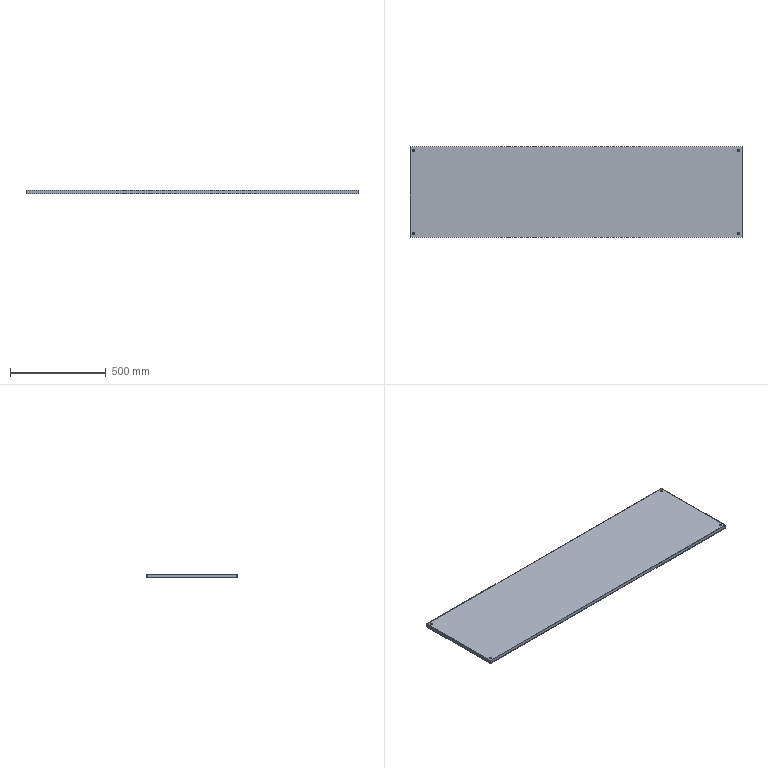Part | SolidWorks | features Extrusion 1, HoleWzd 1, ICE 1, Shell 1 | 1 solid | 32 faces | box 1736 x 471 x 20 mm | volume 1948630 mm3 | cylinder 16 | plane 16 | commonest cylinder face diameters 6.6 x8 11 x8
STEP:
#1=CARTESIAN_POINT('',(-844.5,218.5,18.));
#2=VERTEX_POINT('',#1);
#3=CARTESIAN_POINT('',(-855.5,218.5,18.));
#4=VERTEX_POINT('',#3);
#5=CARTESIAN_POINT('',(-850.,218.5,18.));
#6=DIRECTION('',(0.,0.,-1.));
#7=DIRECTION('',(-1.,0.,0.));
#8=AXIS2_PLACEMENT_3D('',#5,#6,#7);
#9=CIRCLE('',#8,5.5);
#10=EDGE_CURVE('',#2,#4,#9,.T.);
#11=ORIENTED_EDGE('',*,*,#10,.T.);
#12=CARTESIAN_POINT('',(-855.5,218.5,20.));
#13=VERTEX_POINT('',#12);
#14=CARTESIAN_POINT('',(-855.5,218.5,20.));
#15=DIRECTION('',(0.,0.,1.));
#16=VECTOR('',#15,1000.);
#17=LINE('',#14,#16);
#18=EDGE_CURVE('',#4,#13,#17,.T.);
#19=ORIENTED_EDGE('',*,*,#18,.T.);
#20=CARTESIAN_POINT('',(-844.5,218.5,20.));
#21=VERTEX_POINT('',#20);
#22=CARTESIAN_POINT('',(-850.,218.5,20.));
#23=DIRECTION('',(0.,0.,1.));
#24=DIRECTION('',(1.,0.,0.));
#25=AXIS2_PLACEMENT_3D('',#22,#23,#24);
#26=CIRCLE('',#25,5.5);
#27=EDGE_CURVE('',#13,#21,#26,.T.);
#28=ORIENTED_EDGE('',*,*,#27,.T.);
#29=CARTESIAN_POINT('',(-844.5,218.5,20.));
#30=DIRECTION('',(0.,0.,1.));
#31=VECTOR('',#30,1000.);
#32=LINE('',#29,#31);
#33=EDGE_CURVE('',#2,#21,#32,.T.);
#34=ORIENTED_EDGE('',*,*,#33,.F.);
#35=EDGE_LOOP('',(#11,#19,#28,#34));
#36=FACE_OUTER_BOUND('',#35,.T.);
#37=CARTESIAN_POINT('',(-850.,218.5,20.));
#38=DIRECTION('',(0.,0.,1.));
#39=DIRECTION('',(1.,0.,0.));
#40=AXIS2_PLACEMENT_3D('',#37,#38,#39);
#41=CYLINDRICAL_SURFACE('',#40,5.5);
#42=ADVANCED_FACE('',(#36),#41,.F.);
#43=CARTESIAN_POINT('',(-853.3,218.5,0.));
#44=VERTEX_POINT('',#43);
#45=CARTESIAN_POINT('',(-846.7,218.5,0.));
#46=VERTEX_POINT('',#45);
#47=CARTESIAN_POINT('',(-850.,218.5,0.));
#48=DIRECTION('',(0.,0.,1.));
#49=DIRECTION('',(1.,0.,0.));
#50=AXIS2_PLACEMENT_3D('',#47,#48,#49);
#51=CIRCLE('',#50,3.3);
#52=EDGE_CURVE('',#44,#46,#51,.T.);
#53=ORIENTED_EDGE('',*,*,#52,.F.);
#54=CARTESIAN_POINT('',(-853.3,218.5,2.));
#55=VERTEX_POINT('',#54);
#56=CARTESIAN_POINT('',(-853.3,218.5,20.));
#57=DIRECTION('',(0.,0.,1.));
#58=VECTOR('',#57,1000.);
#59=LINE('',#56,#58);
#60=EDGE_CURVE('',#44,#55,#59,.T.);
#61=ORIENTED_EDGE('',*,*,#60,.T.);
#62=CARTESIAN_POINT('',(-846.7,218.5,2.));
#63=VERTEX_POINT('',#62);
#64=CARTESIAN_POINT('',(-850.,218.5,2.));
#65=DIRECTION('',(0.,0.,-1.));
#66=DIRECTION('',(-1.,0.,0.));
#67=AXIS2_PLACEMENT_3D('',#64,#65,#66);
#68=CIRCLE('',#67,3.3);
#69=EDGE_CURVE('',#63,#55,#68,.T.);
#70=ORIENTED_EDGE('',*,*,#69,.F.);
#71=CARTESIAN_POINT('',(-846.7,218.5,20.));
#72=DIRECTION('',(0.,0.,1.));
#73=VECTOR('',#72,1000.);
#74=LINE('',#71,#73);
#75=EDGE_CURVE('',#46,#63,#74,.T.);
#76=ORIENTED_EDGE('',*,*,#75,.F.);
#77=EDGE_LOOP('',(#53,#61,#70,#76));
#78=FACE_OUTER_BOUND('',#77,.T.);
#79=CARTESIAN_POINT('',(-850.,218.5,20.));
#80=DIRECTION('',(0.,0.,1.));
#81=DIRECTION('',(1.,0.,0.));
#82=AXIS2_PLACEMENT_3D('',#79,#80,#81);
#83=CYLINDRICAL_SURFACE('',#82,3.3);
#84=ADVANCED_FACE('',(#78),#83,.F.);
#85=CARTESIAN_POINT('',(-844.5,-218.5,18.));
#86=VERTEX_POINT('',#85);
#87=CARTESIAN_POINT('',(-855.5,-218.5,18.));
#88=VERTEX_POINT('',#87);
#89=CARTESIAN_POINT('',(-850.,-218.5,18.));
#90=DIRECTION('',(0.,0.,-1.));
#91=DIRECTION('',(-1.,0.,0.));
#92=AXIS2_PLACEMENT_3D('',#89,#90,#91);
#93=CIRCLE('',#92,5.5);
#94=EDGE_CURVE('',#86,#88,#93,.T.);
#95=ORIENTED_EDGE('',*,*,#94,.T.);
#96=CARTESIAN_POINT('',(-855.5,-218.5,20.));
#97=VERTEX_POINT('',#96);
#98=CARTESIAN_POINT('',(-855.5,-218.5,20.));
#99=DIRECTION('',(0.,0.,1.));
#100=VECTOR('',#99,1000.);
#101=LINE('',#98,#100);
#102=EDGE_CURVE('',#88,#97,#101,.T.);
#103=ORIENTED_EDGE('',*,*,#102,.T.);
#104=CARTESIAN_POINT('',(-844.5,-218.5,20.));
#105=VERTEX_POINT('',#104);
#106=CARTESIAN_POINT('',(-850.,-218.5,20.));
#107=DIRECTION('',(0.,0.,1.));
#108=DIRECTION('',(1.,0.,0.));
#109=AXIS2_PLACEMENT_3D('',#106,#107,#108);
#110=CIRCLE('',#109,5.5);
#111=EDGE_CURVE('',#97,#105,#110,.T.);
#112=ORIENTED_EDGE('',*,*,#111,.T.);
#113=CARTESIAN_POINT('',(-844.5,-218.5,20.));
#114=DIRECTION('',(0.,0.,1.));
#115=VECTOR('',#114,1000.);
#116=LINE('',#113,#115);
#117=EDGE_CURVE('',#86,#105,#116,.T.);
#118=ORIENTED_EDGE('',*,*,#117,.F.);
#119=EDGE_LOOP('',(#95,#103,#112,#118));
#120=FACE_OUTER_BOUND('',#119,.T.);
#121=CARTESIAN_POINT('',(-850.,-218.5,20.));
#122=DIRECTION('',(0.,0.,1.));
#123=DIRECTION('',(1.,0.,0.));
#124=AXIS2_PLACEMENT_3D('',#121,#122,#123);
#125=CYLINDRICAL_SURFACE('',#124,5.5);
#126=ADVANCED_FACE('',(#120),#125,.F.);
#127=CARTESIAN_POINT('',(-853.3,-218.5,0.));
#128=VERTEX_POINT('',#127);
#129=CARTESIAN_POINT('',(-846.7,-218.5,0.));
#130=VERTEX_POINT('',#129);
#131=CARTESIAN_POINT('',(-850.,-218.5,0.));
#132=DIRECTION('',(0.,0.,1.));
#133=DIRECTION('',(1.,0.,0.));
#134=AXIS2_PLACEMENT_3D('',#131,#132,#133);
#135=CIRCLE('',#134,3.3);
#136=EDGE_CURVE('',#128,#130,#135,.T.);
#137=ORIENTED_EDGE('',*,*,#136,.F.);
#138=CARTESIAN_POINT('',(-853.3,-218.5,2.));
#139=VERTEX_POINT('',#138);
#140=CARTESIAN_POINT('',(-853.3,-218.5,20.));
#141=DIRECTION('',(0.,0.,1.));
#142=VECTOR('',#141,1000.);
#143=LINE('',#140,#142);
#144=EDGE_CURVE('',#128,#139,#143,.T.);
#145=ORIENTED_EDGE('',*,*,#144,.T.);
#146=CARTESIAN_POINT('',(-846.7,-218.5,2.));
#147=VERTEX_POINT('',#146);
#148=CARTESIAN_POINT('',(-850.,-218.5,2.));
#149=DIRECTION('',(0.,0.,-1.));
#150=DIRECTION('',(-1.,0.,0.));
#151=AXIS2_PLACEMENT_3D('',#148,#149,#150);
#152=CIRCLE('',#151,3.3);
#153=EDGE_CURVE('',#147,#139,#152,.T.);
#154=ORIENTED_EDGE('',*,*,#153,.F.);
#155=CARTESIAN_POINT('',(-846.7,-218.5,20.));
#156=DIRECTION('',(0.,0.,1.));
#157=VECTOR('',#156,1000.);
#158=LINE('',#155,#157);
#159=EDGE_CURVE('',#130,#147,#158,.T.);
#160=ORIENTED_EDGE('',*,*,#159,.F.);
#161=EDGE_LOOP('',(#137,#145,#154,#160));
#162=FACE_OUTER_BOUND('',#161,.T.);
#163=CARTESIAN_POINT('',(-850.,-218.5,20.));
#164=DIRECTION('',(0.,0.,1.));
#165=DIRECTION('',(1.,0.,0.));
#166=AXIS2_PLACEMENT_3D('',#163,#164,#165);
#167=CYLINDRICAL_SURFACE('',#166,3.3);
#168=ADVANCED_FACE('',(#162),#167,.F.);
#169=CARTESIAN_POINT('',(855.5,-218.5,18.));
#170=VERTEX_POINT('',#169);
#171=CARTESIAN_POINT('',(844.5,-218.5,18.));
#172=VERTEX_POINT('',#171);
#173=CARTESIAN_POINT('',(850.,-218.5,18.));
#174=DIRECTION('',(0.,0.,-1.));
#175=DIRECTION('',(-1.,0.,0.));
#176=AXIS2_PLACEMENT_3D('',#173,#174,#175);
#177=CIRCLE('',#176,5.5);
#178=EDGE_CURVE('',#170,#172,#177,.T.);
#179=ORIENTED_EDGE('',*,*,#178,.T.);
#180=CARTESIAN_POINT('',(844.5,-218.5,20.));
#181=VERTEX_POINT('',#180);
#182=CARTESIAN_POINT('',(844.5,-218.5,20.));
#183=DIRECTION('',(0.,0.,1.));
#184=VECTOR('',#183,1000.);
#185=LINE('',#182,#184);
#186=EDGE_CURVE('',#172,#181,#185,.T.);
#187=ORIENTED_EDGE('',*,*,#186,.T.);
#188=CARTESIAN_POINT('',(855.5,-218.5,20.));
#189=VERTEX_POINT('',#188);
#190=CARTESIAN_POINT('',(850.,-218.5,20.));
#191=DIRECTION('',(0.,0.,1.));
#192=DIRECTION('',(1.,0.,0.));
#193=AXIS2_PLACEMENT_3D('',#190,#191,#192);
#194=CIRCLE('',#193,5.5);
#195=EDGE_CURVE('',#181,#189,#194,.T.);
#196=ORIENTED_EDGE('',*,*,#195,.T.);
#197=CARTESIAN_POINT('',(855.5,-218.5,20.));
#198=DIRECTION('',(0.,0.,1.));
#199=VECTOR('',#198,1000.);
#200=LINE('',#197,#199);
#201=EDGE_CURVE('',#170,#189,#200,.T.);
#202=ORIENTED_EDGE('',*,*,#201,.F.);
#203=EDGE_LOOP('',(#179,#187,#196,#202));
#204=FACE_OUTER_BOUND('',#203,.T.);
#205=CARTESIAN_POINT('',(850.,-218.5,20.));
#206=DIRECTION('',(0.,0.,1.));
#207=DIRECTION('',(1.,0.,0.));
#208=AXIS2_PLACEMENT_3D('',#205,#206,#207);
#209=CYLINDRICAL_SURFACE('',#208,5.5);
#210=ADVANCED_FACE('',(#204),#209,.F.);
#211=CARTESIAN_POINT('',(846.7,-218.5,0.));
#212=VERTEX_POINT('',#211);
#213=CARTESIAN_POINT('',(853.3,-218.5,0.));
#214=VERTEX_POINT('',#213);
#215=CARTESIAN_POINT('',(850.,-218.5,0.));
#216=DIRECTION('',(0.,0.,1.));
#217=DIRECTION('',(1.,0.,0.));
#218=AXIS2_PLACEMENT_3D('',#215,#216,#217);
#219=CIRCLE('',#218,3.3);
#220=EDGE_CURVE('',#212,#214,#219,.T.);
#221=ORIENTED_EDGE('',*,*,#220,.F.);
#222=CARTESIAN_POINT('',(846.7,-218.5,2.));
#223=VERTEX_POINT('',#222);
#224=CARTESIAN_POINT('',(846.7,-218.5,20.));
#225=DIRECTION('',(0.,0.,1.));
#226=VECTOR('',#225,1000.);
#227=LINE('',#224,#226);
#228=EDGE_CURVE('',#212,#223,#227,.T.);
#229=ORIENTED_EDGE('',*,*,#228,.T.);
#230=CARTESIAN_POINT('',(853.3,-218.5,2.));
#231=VERTEX_POINT('',#230);
#232=CARTESIAN_POINT('',(850.,-218.5,2.));
#233=DIRECTION('',(0.,0.,-1.));
#234=DIRECTION('',(-1.,0.,0.));
#235=AXIS2_PLACEMENT_3D('',#232,#233,#234);
#236=CIRCLE('',#235,3.3);
#237=EDGE_CURVE('',#231,#223,#236,.T.);
#238=ORIENTED_EDGE('',*,*,#237,.F.);
#239=CARTESIAN_POINT('',(853.3,-218.5,20.));
#240=DIRECTION('',(0.,0.,1.));
#241=VECTOR('',#240,1000.);
#242=LINE('',#239,#241);
#243=EDGE_CURVE('',#214,#231,#242,.T.);
#244=ORIENTED_EDGE('',*,*,#243,.F.);
#245=EDGE_LOOP('',(#221,#229,#238,#244));
#246=FACE_OUTER_BOUND('',#245,.T.);
#247=CARTESIAN_POINT('',(850.,-218.5,20.));
#248=DIRECTION('',(0.,0.,1.));
#249=DIRECTION('',(1.,0.,0.));
#250=AXIS2_PLACEMENT_3D('',#247,#248,#249);
#251=CYLINDRICAL_SURFACE('',#250,3.3);
#252=ADVANCED_FACE('',(#246),#251,.F.);
#253=CARTESIAN_POINT('',(855.5,218.5,18.));
#254=VERTEX_POINT('',#253);
#255=CARTESIAN_POINT('',(844.5,218.5,18.));
#256=VERTEX_POINT('',#255);
#257=CARTESIAN_POINT('',(850.,218.5,18.));
#258=DIRECTION('',(0.,0.,-1.));
#259=DIRECTION('',(-1.,0.,0.));
#260=AXIS2_PLACEMENT_3D('',#257,#258,#259);
#261=CIRCLE('',#260,5.5);
#262=EDGE_CURVE('',#254,#256,#261,.T.);
#263=ORIENTED_EDGE('',*,*,#262,.T.);
#264=CARTESIAN_POINT('',(844.5,218.5,20.));
#265=VERTEX_POINT('',#264);
#266=CARTESIAN_POINT('',(844.5,218.5,20.));
#267=DIRECTION('',(0.,0.,1.));
#268=VECTOR('',#267,1000.);
#269=LINE('',#266,#268);
#270=EDGE_CURVE('',#256,#265,#269,.T.);
#271=ORIENTED_EDGE('',*,*,#270,.T.);
#272=CARTESIAN_POINT('',(855.5,218.5,20.));
#273=VERTEX_POINT('',#272);
#274=CARTESIAN_POINT('',(850.,218.5,20.));
#275=DIRECTION('',(0.,0.,1.));
#276=DIRECTION('',(1.,0.,0.));
#277=AXIS2_PLACEMENT_3D('',#274,#275,#276);
#278=CIRCLE('',#277,5.5);
#279=EDGE_CURVE('',#265,#273,#278,.T.);
#280=ORIENTED_EDGE('',*,*,#279,.T.);
#281=CARTESIAN_POINT('',(855.5,218.5,20.));
#282=DIRECTION('',(0.,0.,1.));
#283=VECTOR('',#282,1000.);
#284=LINE('',#281,#283);
#285=EDGE_CURVE('',#254,#273,#284,.T.);
#286=ORIENTED_EDGE('',*,*,#285,.F.);
#287=EDGE_LOOP('',(#263,#271,#280,#286));
#288=FACE_OUTER_BOUND('',#287,.T.);
#289=CARTESIAN_POINT('',(850.,218.5,20.));
#290=DIRECTION('',(0.,0.,1.));
#291=DIRECTION('',(1.,0.,0.));
#292=AXIS2_PLACEMENT_3D('',#289,#290,#291);
#293=CYLINDRICAL_SURFACE('',#292,5.5);
#294=ADVANCED_FACE('',(#288),#293,.F.);
#295=CARTESIAN_POINT('',(846.7,218.5,0.));
#296=VERTEX_POINT('',#295);
#297=CARTESIAN_POINT('',(853.3,218.5,0.));
#298=VERTEX_POINT('',#297);
#299=CARTESIAN_POINT('',(850.,218.5,0.));
#300=DIRECTION('',(0.,0.,1.));
#301=DIRECTION('',(1.,0.,0.));
#302=AXIS2_PLACEMENT_3D('',#299,#300,#301);
#303=CIRCLE('',#302,3.3);
#304=EDGE_CURVE('',#296,#298,#303,.T.);
#305=ORIENTED_EDGE('',*,*,#304,.F.);
#306=CARTESIAN_POINT('',(846.7,218.5,2.));
#307=VERTEX_POINT('',#306);
#308=CARTESIAN_POINT('',(846.7,218.5,20.));
#309=DIRECTION('',(0.,0.,1.));
#310=VECTOR('',#309,1000.);
#311=LINE('',#308,#310);
#312=EDGE_CURVE('',#296,#307,#311,.T.);
#313=ORIENTED_EDGE('',*,*,#312,.T.);
#314=CARTESIAN_POINT('',(853.3,218.5,2.));
#315=VERTEX_POINT('',#314);
#316=CARTESIAN_POINT('',(850.,218.5,2.));
#317=DIRECTION('',(0.,0.,-1.));
#318=DIRECTION('',(-1.,0.,0.));
#319=AXIS2_PLACEMENT_3D('',#316,#317,#318);
#320=CIRCLE('',#319,3.3);
#321=EDGE_CURVE('',#315,#307,#320,.T.);
#322=ORIENTED_EDGE('',*,*,#321,.F.);
#323=CARTESIAN_POINT('',(853.3,218.5,20.));
#324=DIRECTION('',(0.,0.,1.));
#325=VECTOR('',#324,1000.);
#326=LINE('',#323,#325);
#327=EDGE_CURVE('',#298,#315,#326,.T.);
#328=ORIENTED_EDGE('',*,*,#327,.F.);
#329=EDGE_LOOP('',(#305,#313,#322,#328));
#330=FACE_OUTER_BOUND('',#329,.T.);
#331=CARTESIAN_POINT('',(850.,218.5,20.));
#332=DIRECTION('',(0.,0.,1.));
#333=DIRECTION('',(1.,0.,0.));
#334=AXIS2_PLACEMENT_3D('',#331,#332,#333);
#335=CYLINDRICAL_SURFACE('',#334,3.3);
#336=ADVANCED_FACE('',(#330),#335,.F.);
#337=CARTESIAN_POINT('',(-850.,218.5,0.));
#338=DIRECTION('',(0.,0.,1.));
#339=DIRECTION('',(1.,0.,0.));
#340=AXIS2_PLACEMENT_3D('',#337,#338,#339);
#341=CIRCLE('',#340,3.3);
#342=EDGE_CURVE('',#46,#44,#341,.T.);
#343=ORIENTED_EDGE('',*,*,#342,.T.);
#344=ORIENTED_EDGE('',*,*,#52,.T.);
#345=EDGE_LOOP('',(#343,#344));
#346=FACE_BOUND('',#345,.T.);
#347=CARTESIAN_POINT('',(-850.,-218.5,0.));
#348=DIRECTION('',(0.,0.,1.));
#349=DIRECTION('',(1.,0.,0.));
#350=AXIS2_PLACEMENT_3D('',#347,#348,#349);
#351=CIRCLE('',#350,3.3);
#352=EDGE_CURVE('',#130,#128,#351,.T.);
#353=ORIENTED_EDGE('',*,*,#352,.T.);
#354=ORIENTED_EDGE('',*,*,#136,.T.);
#355=EDGE_LOOP('',(#353,#354));
#356=FACE_BOUND('',#355,.T.);
#357=CARTESIAN_POINT('',(850.,-218.5,0.));
#358=DIRECTION('',(0.,0.,1.));
#359=DIRECTION('',(1.,0.,0.));
#360=AXIS2_PLACEMENT_3D('',#357,#358,#359);
#361=CIRCLE('',#360,3.3);
#362=EDGE_CURVE('',#214,#212,#361,.T.);
#363=ORIENTED_EDGE('',*,*,#362,.T.);
#364=ORIENTED_EDGE('',*,*,#220,.T.);
#365=EDGE_LOOP('',(#363,#364));
#366=FACE_BOUND('',#365,.T.);
#367=CARTESIAN_POINT('',(850.,218.5,0.));
#368=DIRECTION('',(0.,0.,1.));
#369=DIRECTION('',(1.,0.,0.));
#370=AXIS2_PLACEMENT_3D('',#367,#368,#369);
#371=CIRCLE('',#370,3.3);
#372=EDGE_CURVE('',#298,#296,#371,.T.);
#373=ORIENTED_EDGE('',*,*,#372,.T.);
#374=ORIENTED_EDGE('',*,*,#304,.T.);
#375=EDGE_LOOP('',(#373,#374));
#376=FACE_BOUND('',#375,.T.);
#377=CARTESIAN_POINT('',(868.,-235.5,0.));
#378=VERTEX_POINT('',#377);
#379=CARTESIAN_POINT('',(868.,235.5,0.));
#380=VERTEX_POINT('',#379);
#381=CARTESIAN_POINT('',(868.,-235.5,0.));
#382=DIRECTION('',(0.,1.,0.));
#383=VECTOR('',#382,1000.);
#384=LINE('',#381,#383);
#385=EDGE_CURVE('',#378,#380,#384,.T.);
#386=ORIENTED_EDGE('',*,*,#385,.F.);
#387=CARTESIAN_POINT('',(-868.,-235.5,0.));
#388=VERTEX_POINT('',#387);
#389=CARTESIAN_POINT('',(-868.,-235.5,0.));
#390=DIRECTION('',(1.,0.,0.));
#391=VECTOR('',#390,1000.);
#392=LINE('',#389,#391);
#393=EDGE_CURVE('',#388,#378,#392,.T.);
#394=ORIENTED_EDGE('',*,*,#393,.F.);
#395=CARTESIAN_POINT('',(-868.,235.5,0.));
#396=VERTEX_POINT('',#395);
#397=CARTESIAN_POINT('',(-868.,-235.5,0.));
#398=DIRECTION('',(0.,-1.,0.));
#399=VECTOR('',#398,1000.);
#400=LINE('',#397,#399);
#401=EDGE_CURVE('',#396,#388,#400,.T.);
#402=ORIENTED_EDGE('',*,*,#401,.F.);
#403=CARTESIAN_POINT('',(-868.,235.5,0.));
#404=DIRECTION('',(-1.,0.,0.));
#405=VECTOR('',#404,1000.);
#406=LINE('',#403,#405);
#407=EDGE_CURVE('',#380,#396,#406,.T.);
#408=ORIENTED_EDGE('',*,*,#407,.F.);
#409=EDGE_LOOP('',(#386,#394,#402,#408));
#410=FACE_OUTER_BOUND('',#409,.T.);
#411=CARTESIAN_POINT('',(848.,-215.5,0.));
#412=VERTEX_POINT('',#411);
#413=CARTESIAN_POINT('',(-848.,-215.5,0.));
#414=VERTEX_POINT('',#413);
#415=CARTESIAN_POINT('',(848.,-215.5,0.));
#416=DIRECTION('',(-1.,0.,0.));
#417=VECTOR('',#416,1000.);
#418=LINE('',#415,#417);
#419=EDGE_CURVE('',#412,#414,#418,.T.);
#420=ORIENTED_EDGE('',*,*,#419,.F.);
#421=CARTESIAN_POINT('',(848.,215.5,0.));
#422=VERTEX_POINT('',#421);
#423=CARTESIAN_POINT('',(848.,-215.5,0.));
#424=DIRECTION('',(0.,1.,0.));
#425=VECTOR('',#424,1000.);
#426=LINE('',#423,#425);
#427=EDGE_CURVE('',#412,#422,#426,.T.);
#428=ORIENTED_EDGE('',*,*,#427,.T.);
#429=CARTESIAN_POINT('',(-848.,215.5,0.));
#430=VERTEX_POINT('',#429);
#431=CARTESIAN_POINT('',(848.,215.5,0.));
#432=DIRECTION('',(-1.,0.,0.));
#433=VECTOR('',#432,1000.);
#434=LINE('',#431,#433);
#435=EDGE_CURVE('',#422,#430,#434,.T.);
#436=ORIENTED_EDGE('',*,*,#435,.T.);
#437=CARTESIAN_POINT('',(-848.,-215.5,0.));
#438=DIRECTION('',(0.,1.,0.));
#439=VECTOR('',#438,1000.);
#440=LINE('',#437,#439);
#441=EDGE_CURVE('',#414,#430,#440,.T.);
#442=ORIENTED_EDGE('',*,*,#441,.F.);
#443=EDGE_LOOP('',(#420,#428,#436,#442));
#444=FACE_BOUND('',#443,.T.);
#445=CARTESIAN_POINT('',(0.,0.,0.));
#446=DIRECTION('',(0.,0.,-1.));
#447=DIRECTION('',(-1.,0.,0.));
#448=AXIS2_PLACEMENT_3D('',#445,#446,#447);
#449=PLANE('',#448);
#450=ADVANCED_FACE('',(#346,#356,#366,#376,#410,#444),#449,.T.);
#451=ORIENTED_EDGE('',*,*,#385,.T.);
#452=CARTESIAN_POINT('',(868.,235.5,20.));
#453=VERTEX_POINT('',#452);
#454=CARTESIAN_POINT('',(868.,235.5,20.));
#455=DIRECTION('',(0.,0.,-1.));
#456=VECTOR('',#455,1000.);
#457=LINE('',#454,#456);
#458=EDGE_CURVE('',#453,#380,#457,.T.);
#459=ORIENTED_EDGE('',*,*,#458,.F.);
#460=CARTESIAN_POINT('',(868.,-235.5,20.));
#461=VERTEX_POINT('',#460);
#462=CARTESIAN_POINT('',(868.,-235.5,20.));
#463=DIRECTION('',(0.,1.,0.));
#464=VECTOR('',#463,1000.);
#465=LINE('',#462,#464);
#466=EDGE_CURVE('',#461,#453,#465,.T.);
#467=ORIENTED_EDGE('',*,*,#466,.F.);
#468=CARTESIAN_POINT('',(868.,-235.5,20.));
#469=DIRECTION('',(0.,0.,-1.));
#470=VECTOR('',#469,1000.);
#471=LINE('',#468,#470);
#472=EDGE_CURVE('',#461,#378,#471,.T.);
#473=ORIENTED_EDGE('',*,*,#472,.T.);
#474=EDGE_LOOP('',(#451,#459,#467,#473));
#475=FACE_OUTER_BOUND('',#474,.T.);
#476=CARTESIAN_POINT('',(868.,-235.5,20.));
#477=DIRECTION('',(-1.,0.,0.));
#478=DIRECTION('',(0.,0.,1.));
#479=AXIS2_PLACEMENT_3D('',#476,#477,#478);
#480=PLANE('',#479);
#481=ADVANCED_FACE('',(#475),#480,.F.);
#482=ORIENTED_EDGE('',*,*,#407,.T.);
#483=CARTESIAN_POINT('',(-868.,235.5,20.));
#484=VERTEX_POINT('',#483);
#485=CARTESIAN_POINT('',(-868.,235.5,20.));
#486=DIRECTION('',(0.,0.,-1.));
#487=VECTOR('',#486,1000.);
#488=LINE('',#485,#487);
#489=EDGE_CURVE('',#484,#396,#488,.T.);
#490=ORIENTED_EDGE('',*,*,#489,.F.);
#491=CARTESIAN_POINT('',(-868.,235.5,20.));
#492=DIRECTION('',(-1.,0.,0.));
#493=VECTOR('',#492,1000.);
#494=LINE('',#491,#493);
#495=EDGE_CURVE('',#453,#484,#494,.T.);
#496=ORIENTED_EDGE('',*,*,#495,.F.);
#497=ORIENTED_EDGE('',*,*,#458,.T.);
#498=EDGE_LOOP('',(#482,#490,#496,#497));
#499=FACE_OUTER_BOUND('',#498,.T.);
#500=CARTESIAN_POINT('',(-868.,235.5,20.));
#501=DIRECTION('',(0.,-1.,0.));
#502=DIRECTION('',(0.,0.,-1.));
#503=AXIS2_PLACEMENT_3D('',#500,#501,#502);
#504=PLANE('',#503);
#505=ADVANCED_FACE('',(#499),#504,.F.);
#506=ORIENTED_EDGE('',*,*,#401,.T.);
#507=CARTESIAN_POINT('',(-868.,-235.5,20.));
#508=VERTEX_POINT('',#507);
#509=CARTESIAN_POINT('',(-868.,-235.5,20.));
#510=DIRECTION('',(0.,0.,-1.));
#511=VECTOR('',#510,1000.);
#512=LINE('',#509,#511);
#513=EDGE_CURVE('',#508,#388,#512,.T.);
#514=ORIENTED_EDGE('',*,*,#513,.F.);
#515=CARTESIAN_POINT('',(-868.,-235.5,20.));
#516=DIRECTION('',(0.,-1.,0.));
#517=VECTOR('',#516,1000.);
#518=LINE('',#515,#517);
#519=EDGE_CURVE('',#484,#508,#518,.T.);
#520=ORIENTED_EDGE('',*,*,#519,.F.);
#521=ORIENTED_EDGE('',*,*,#489,.T.);
#522=EDGE_LOOP('',(#506,#514,#520,#521));
#523=FACE_OUTER_BOUND('',#522,.T.);
#524=CARTESIAN_POINT('',(-868.,-235.5,20.));
#525=DIRECTION('',(1.,0.,0.));
#526=DIRECTION('',(0.,0.,-1.));
#527=AXIS2_PLACEMENT_3D('',#524,#525,#526);
#528=PLANE('',#527);
#529=ADVANCED_FACE('',(#523),#528,.F.);
#530=ORIENTED_EDGE('',*,*,#393,.T.);
#531=ORIENTED_EDGE('',*,*,#472,.F.);
#532=CARTESIAN_POINT('',(-868.,-235.5,20.));
#533=DIRECTION('',(1.,0.,0.));
#534=VECTOR('',#533,1000.);
#535=LINE('',#532,#534);
#536=EDGE_CURVE('',#508,#461,#535,.T.);
#537=ORIENTED_EDGE('',*,*,#536,.F.);
#538=ORIENTED_EDGE('',*,*,#513,.T.);
#539=EDGE_LOOP('',(#530,#531,#537,#538));
#540=FACE_OUTER_BOUND('',#539,.T.);
#541=CARTESIAN_POINT('',(-868.,-235.5,20.));
#542=DIRECTION('',(0.,1.,0.));
#543=DIRECTION('',(0.,0.,1.));
#544=AXIS2_PLACEMENT_3D('',#541,#542,#543);
#545=PLANE('',#544);
#546=ADVANCED_FACE('',(#540),#545,.F.);
#547=CARTESIAN_POINT('',(-850.,218.5,20.));
#548=DIRECTION('',(0.,0.,1.));
#549=DIRECTION('',(1.,0.,0.));
#550=AXIS2_PLACEMENT_3D('',#547,#548,#549);
#551=CIRCLE('',#550,5.5);
#552=EDGE_CURVE('',#21,#13,#551,.T.);
#553=ORIENTED_EDGE('',*,*,#552,.F.);
#554=ORIENTED_EDGE('',*,*,#27,.F.);
#555=EDGE_LOOP('',(#553,#554));
#556=FACE_BOUND('',#555,.T.);
#557=CARTESIAN_POINT('',(-850.,-218.5,20.));
#558=DIRECTION('',(0.,0.,1.));
#559=DIRECTION('',(1.,0.,0.));
#560=AXIS2_PLACEMENT_3D('',#557,#558,#559);
#561=CIRCLE('',#560,5.5);
#562=EDGE_CURVE('',#105,#97,#561,.T.);
#563=ORIENTED_EDGE('',*,*,#562,.F.);
#564=ORIENTED_EDGE('',*,*,#111,.F.);
#565=EDGE_LOOP('',(#563,#564));
#566=FACE_BOUND('',#565,.T.);
#567=CARTESIAN_POINT('',(850.,-218.5,20.));
#568=DIRECTION('',(0.,0.,1.));
#569=DIRECTION('',(1.,0.,0.));
#570=AXIS2_PLACEMENT_3D('',#567,#568,#569);
#571=CIRCLE('',#570,5.5);
#572=EDGE_CURVE('',#189,#181,#571,.T.);
#573=ORIENTED_EDGE('',*,*,#572,.F.);
#574=ORIENTED_EDGE('',*,*,#195,.F.);
#575=EDGE_LOOP('',(#573,#574));
#576=FACE_BOUND('',#575,.T.);
#577=CARTESIAN_POINT('',(850.,218.5,20.));
#578=DIRECTION('',(0.,0.,1.));
#579=DIRECTION('',(1.,0.,0.));
#580=AXIS2_PLACEMENT_3D('',#577,#578,#579);
#581=CIRCLE('',#580,5.5);
#582=EDGE_CURVE('',#273,#265,#581,.T.);
#583=ORIENTED_EDGE('',*,*,#582,.F.);
#584=ORIENTED_EDGE('',*,*,#279,.F.);
#585=EDGE_LOOP('',(#583,#584));
#586=FACE_BOUND('',#585,.T.);
#587=ORIENTED_EDGE('',*,*,#466,.T.);
#588=ORIENTED_EDGE('',*,*,#495,.T.);
#589=ORIENTED_EDGE('',*,*,#519,.T.);
#590=ORIENTED_EDGE('',*,*,#536,.T.);
#591=EDGE_LOOP('',(#587,#588,#589,#590));
#592=FACE_OUTER_BOUND('',#591,.T.);
#593=CARTESIAN_POINT('',(0.,0.,20.));
#594=DIRECTION('',(0.,0.,-1.));
#595=DIRECTION('',(-1.,0.,0.));
#596=AXIS2_PLACEMENT_3D('',#593,#594,#595);
#597=PLANE('',#596);
#598=ADVANCED_FACE('',(#556,#566,#576,#586,#592),#597,.F.);
#599=ORIENTED_EDGE('',*,*,#427,.F.);
#600=CARTESIAN_POINT('',(848.,-215.5,2.));
#601=VERTEX_POINT('',#600);
#602=CARTESIAN_POINT('',(848.,-215.5,2.));
#603=DIRECTION('',(0.,0.,-1.));
#604=VECTOR('',#603,1000.);
#605=LINE('',#602,#604);
#606=EDGE_CURVE('',#601,#412,#605,.T.);
#607=ORIENTED_EDGE('',*,*,#606,.F.);
#608=CARTESIAN_POINT('',(848.,215.5,2.));
#609=VERTEX_POINT('',#608);
#610=CARTESIAN_POINT('',(848.,-215.5,2.));
#611=DIRECTION('',(0.,1.,0.));
#612=VECTOR('',#611,1000.);
#613=LINE('',#610,#612);
#614=EDGE_CURVE('',#601,#609,#613,.T.);
#615=ORIENTED_EDGE('',*,*,#614,.T.);
#616=CARTESIAN_POINT('',(848.,215.5,2.));
#617=DIRECTION('',(0.,0.,-1.));
#618=VECTOR('',#617,1000.);
#619=LINE('',#616,#618);
#620=EDGE_CURVE('',#609,#422,#619,.T.);
#621=ORIENTED_EDGE('',*,*,#620,.T.);
#622=EDGE_LOOP('',(#599,#607,#615,#621));
#623=FACE_OUTER_BOUND('',#622,.T.);
#624=CARTESIAN_POINT('',(848.,-215.5,2.));
#625=DIRECTION('',(-1.,0.,0.));
#626=DIRECTION('',(0.,0.,1.));
#627=AXIS2_PLACEMENT_3D('',#624,#625,#626);
#628=PLANE('',#627);
#629=ADVANCED_FACE('',(#623),#628,.T.);
#630=ORIENTED_EDGE('',*,*,#435,.F.);
#631=ORIENTED_EDGE('',*,*,#620,.F.);
#632=CARTESIAN_POINT('',(-848.,215.5,2.));
#633=VERTEX_POINT('',#632);
#634=CARTESIAN_POINT('',(848.,215.5,2.));
#635=DIRECTION('',(-1.,0.,0.));
#636=VECTOR('',#635,1000.);
#637=LINE('',#634,#636);
#638=EDGE_CURVE('',#609,#633,#637,.T.);
#639=ORIENTED_EDGE('',*,*,#638,.T.);
#640=CARTESIAN_POINT('',(-848.,215.5,2.));
#641=DIRECTION('',(0.,0.,-1.));
#642=VECTOR('',#641,1000.);
#643=LINE('',#640,#642);
#644=EDGE_CURVE('',#633,#430,#643,.T.);
#645=ORIENTED_EDGE('',*,*,#644,.T.);
#646=EDGE_LOOP('',(#630,#631,#639,#645));
#647=FACE_OUTER_BOUND('',#646,.T.);
#648=CARTESIAN_POINT('',(848.,215.5,2.));
#649=DIRECTION('',(0.,-1.,0.));
#650=DIRECTION('',(0.,0.,-1.));
#651=AXIS2_PLACEMENT_3D('',#648,#649,#650);
#652=PLANE('',#651);
#653=ADVANCED_FACE('',(#647),#652,.T.);
#654=ORIENTED_EDGE('',*,*,#441,.T.);
#655=ORIENTED_EDGE('',*,*,#644,.F.);
#656=CARTESIAN_POINT('',(-848.,-215.5,2.));
#657=VERTEX_POINT('',#656);
#658=CARTESIAN_POINT('',(-848.,-215.5,2.));
#659=DIRECTION('',(0.,1.,0.));
#660=VECTOR('',#659,1000.);
#661=LINE('',#658,#660);
#662=EDGE_CURVE('',#657,#633,#661,.T.);
#663=ORIENTED_EDGE('',*,*,#662,.F.);
#664=CARTESIAN_POINT('',(-848.,-215.5,2.));
#665=DIRECTION('',(0.,0.,-1.));
#666=VECTOR('',#665,1000.);
#667=LINE('',#664,#666);
#668=EDGE_CURVE('',#657,#414,#667,.T.);
#669=ORIENTED_EDGE('',*,*,#668,.T.);
#670=EDGE_LOOP('',(#654,#655,#663,#669));
#671=FACE_OUTER_BOUND('',#670,.T.);
#672=CARTESIAN_POINT('',(-848.,-215.5,2.));
#673=DIRECTION('',(-1.,0.,0.));
#674=DIRECTION('',(0.,0.,1.));
#675=AXIS2_PLACEMENT_3D('',#672,#673,#674);
#676=PLANE('',#675);
#677=ADVANCED_FACE('',(#671),#676,.F.);
#678=ORIENTED_EDGE('',*,*,#419,.T.);
#679=ORIENTED_EDGE('',*,*,#668,.F.);
#680=CARTESIAN_POINT('',(848.,-215.5,2.));
#681=DIRECTION('',(-1.,0.,0.));
#682=VECTOR('',#681,1000.);
#683=LINE('',#680,#682);
#684=EDGE_CURVE('',#601,#657,#683,.T.);
#685=ORIENTED_EDGE('',*,*,#684,.F.);
#686=ORIENTED_EDGE('',*,*,#606,.T.);
#687=EDGE_LOOP('',(#678,#679,#685,#686));
#688=FACE_OUTER_BOUND('',#687,.T.);
#689=CARTESIAN_POINT('',(848.,-215.5,2.));
#690=DIRECTION('',(0.,-1.,0.));
#691=DIRECTION('',(0.,0.,-1.));
#692=AXIS2_PLACEMENT_3D('',#689,#690,#691);
#693=PLANE('',#692);
#694=ADVANCED_FACE('',(#688),#693,.F.);
#695=ORIENTED_EDGE('',*,*,#69,.T.);
#696=CARTESIAN_POINT('',(-850.,218.5,2.));
#697=DIRECTION('',(0.,0.,-1.));
#698=DIRECTION('',(-1.,0.,0.));
#699=AXIS2_PLACEMENT_3D('',#696,#697,#698);
#700=CIRCLE('',#699,3.3);
#701=EDGE_CURVE('',#55,#63,#700,.T.);
#702=ORIENTED_EDGE('',*,*,#701,.T.);
#703=EDGE_LOOP('',(#695,#702));
#704=FACE_BOUND('',#703,.T.);
#705=ORIENTED_EDGE('',*,*,#153,.T.);
#706=CARTESIAN_POINT('',(-850.,-218.5,2.));
#707=DIRECTION('',(0.,0.,-1.));
#708=DIRECTION('',(-1.,0.,0.));
#709=AXIS2_PLACEMENT_3D('',#706,#707,#708);
#710=CIRCLE('',#709,3.3);
#711=EDGE_CURVE('',#139,#147,#710,.T.);
#712=ORIENTED_EDGE('',*,*,#711,.T.);
#713=EDGE_LOOP('',(#705,#712));
#714=FACE_BOUND('',#713,.T.);
#715=ORIENTED_EDGE('',*,*,#237,.T.);
#716=CARTESIAN_POINT('',(850.,-218.5,2.));
#717=DIRECTION('',(0.,0.,-1.));
#718=DIRECTION('',(-1.,0.,0.));
#719=AXIS2_PLACEMENT_3D('',#716,#717,#718);
#720=CIRCLE('',#719,3.3);
#721=EDGE_CURVE('',#223,#231,#720,.T.);
#722=ORIENTED_EDGE('',*,*,#721,.T.);
#723=EDGE_LOOP('',(#715,#722));
#724=FACE_BOUND('',#723,.T.);
#725=ORIENTED_EDGE('',*,*,#321,.T.);
#726=CARTESIAN_POINT('',(850.,218.5,2.));
#727=DIRECTION('',(0.,0.,-1.));
#728=DIRECTION('',(-1.,0.,0.));
#729=AXIS2_PLACEMENT_3D('',#726,#727,#728);
#730=CIRCLE('',#729,3.3);
#731=EDGE_CURVE('',#307,#315,#730,.T.);
#732=ORIENTED_EDGE('',*,*,#731,.T.);
#733=EDGE_LOOP('',(#725,#732));
#734=FACE_BOUND('',#733,.T.);
#735=CARTESIAN_POINT('',(866.,-233.5,2.));
#736=VERTEX_POINT('',#735);
#737=CARTESIAN_POINT('',(866.,233.5,2.));
#738=VERTEX_POINT('',#737);
#739=CARTESIAN_POINT('',(866.,0.,2.));
#740=DIRECTION('',(0.,1.,0.));
#741=VECTOR('',#740,1000.);
#742=LINE('',#739,#741);
#743=EDGE_CURVE('',#736,#738,#742,.T.);
#744=ORIENTED_EDGE('',*,*,#743,.T.);
#745=CARTESIAN_POINT('',(-866.,233.5,2.));
#746=VERTEX_POINT('',#745);
#747=CARTESIAN_POINT('',(0.,233.5,2.));
#748=DIRECTION('',(-1.,0.,0.));
#749=VECTOR('',#748,1000.);
#750=LINE('',#747,#749);
#751=EDGE_CURVE('',#738,#746,#750,.T.);
#752=ORIENTED_EDGE('',*,*,#751,.T.);
#753=CARTESIAN_POINT('',(-866.,-233.5,2.));
#754=VERTEX_POINT('',#753);
#755=CARTESIAN_POINT('',(-866.,0.,2.));
#756=DIRECTION('',(0.,-1.,0.));
#757=VECTOR('',#756,1000.);
#758=LINE('',#755,#757);
#759=EDGE_CURVE('',#746,#754,#758,.T.);
#760=ORIENTED_EDGE('',*,*,#759,.T.);
#761=CARTESIAN_POINT('',(0.,-233.5,2.));
#762=DIRECTION('',(1.,0.,0.));
#763=VECTOR('',#762,1000.);
#764=LINE('',#761,#763);
#765=EDGE_CURVE('',#754,#736,#764,.T.);
#766=ORIENTED_EDGE('',*,*,#765,.T.);
#767=EDGE_LOOP('',(#744,#752,#760,#766));
#768=FACE_OUTER_BOUND('',#767,.T.);
#769=ORIENTED_EDGE('',*,*,#684,.T.);
#770=ORIENTED_EDGE('',*,*,#662,.T.);
#771=ORIENTED_EDGE('',*,*,#638,.F.);
#772=ORIENTED_EDGE('',*,*,#614,.F.);
#773=EDGE_LOOP('',(#769,#770,#771,#772));
#774=FACE_BOUND('',#773,.T.);
#775=CARTESIAN_POINT('',(0.,0.,2.));
#776=DIRECTION('',(0.,0.,-1.));
#777=DIRECTION('',(-1.,0.,0.));
#778=AXIS2_PLACEMENT_3D('',#775,#776,#777);
#779=PLANE('',#778);
#780=ADVANCED_FACE('',(#704,#714,#724,#734,#768,#774),#779,.F.);
#781=ORIENTED_EDGE('',*,*,#743,.F.);
#782=CARTESIAN_POINT('',(866.,-233.5,18.));
#783=VERTEX_POINT('',#782);
#784=CARTESIAN_POINT('',(866.,-233.5,20.));
#785=DIRECTION('',(0.,0.,-1.));
#786=VECTOR('',#785,1000.);
#787=LINE('',#784,#786);
#788=EDGE_CURVE('',#783,#736,#787,.T.);
#789=ORIENTED_EDGE('',*,*,#788,.F.);
#790=CARTESIAN_POINT('',(866.,233.5,18.));
#791=VERTEX_POINT('',#790);
#792=CARTESIAN_POINT('',(866.,0.,18.));
#793=DIRECTION('',(0.,1.,0.));
#794=VECTOR('',#793,1000.);
#795=LINE('',#792,#794);
#796=EDGE_CURVE('',#783,#791,#795,.T.);
#797=ORIENTED_EDGE('',*,*,#796,.T.);
#798=CARTESIAN_POINT('',(866.,233.5,20.));
#799=DIRECTION('',(0.,0.,-1.));
#800=VECTOR('',#799,1000.);
#801=LINE('',#798,#800);
#802=EDGE_CURVE('',#791,#738,#801,.T.);
#803=ORIENTED_EDGE('',*,*,#802,.T.);
#804=EDGE_LOOP('',(#781,#789,#797,#803));
#805=FACE_OUTER_BOUND('',#804,.T.);
#806=CARTESIAN_POINT('',(866.,-235.5,20.));
#807=DIRECTION('',(-1.,0.,0.));
#808=DIRECTION('',(0.,0.,1.));
#809=AXIS2_PLACEMENT_3D('',#806,#807,#808);
#810=PLANE('',#809);
#811=ADVANCED_FACE('',(#805),#810,.T.);
#812=ORIENTED_EDGE('',*,*,#751,.F.);
#813=ORIENTED_EDGE('',*,*,#802,.F.);
#814=CARTESIAN_POINT('',(-866.,233.5,18.));
#815=VERTEX_POINT('',#814);
#816=CARTESIAN_POINT('',(0.,233.5,18.));
#817=DIRECTION('',(-1.,0.,0.));
#818=VECTOR('',#817,1000.);
#819=LINE('',#816,#818);
#820=EDGE_CURVE('',#791,#815,#819,.T.);
#821=ORIENTED_EDGE('',*,*,#820,.T.);
#822=CARTESIAN_POINT('',(-866.,233.5,20.));
#823=DIRECTION('',(0.,0.,-1.));
#824=VECTOR('',#823,1000.);
#825=LINE('',#822,#824);
#826=EDGE_CURVE('',#815,#746,#825,.T.);
#827=ORIENTED_EDGE('',*,*,#826,.T.);
#828=EDGE_LOOP('',(#812,#813,#821,#827));
#829=FACE_OUTER_BOUND('',#828,.T.);
#830=CARTESIAN_POINT('',(-868.,233.5,20.));
#831=DIRECTION('',(0.,-1.,0.));
#832=DIRECTION('',(0.,0.,-1.));
#833=AXIS2_PLACEMENT_3D('',#830,#831,#832);
#834=PLANE('',#833);
#835=ADVANCED_FACE('',(#829),#834,.T.);
#836=ORIENTED_EDGE('',*,*,#759,.F.);
#837=ORIENTED_EDGE('',*,*,#826,.F.);
#838=CARTESIAN_POINT('',(-866.,-233.5,18.));
#839=VERTEX_POINT('',#838);
#840=CARTESIAN_POINT('',(-866.,0.,18.));
#841=DIRECTION('',(0.,-1.,0.));
#842=VECTOR('',#841,1000.);
#843=LINE('',#840,#842);
#844=EDGE_CURVE('',#815,#839,#843,.T.);
#845=ORIENTED_EDGE('',*,*,#844,.T.);
#846=CARTESIAN_POINT('',(-866.,-233.5,20.));
#847=DIRECTION('',(0.,0.,-1.));
#848=VECTOR('',#847,1000.);
#849=LINE('',#846,#848);
#850=EDGE_CURVE('',#839,#754,#849,.T.);
#851=ORIENTED_EDGE('',*,*,#850,.T.);
#852=EDGE_LOOP('',(#836,#837,#845,#851));
#853=FACE_OUTER_BOUND('',#852,.T.);
#854=CARTESIAN_POINT('',(-866.,-235.5,20.));
#855=DIRECTION('',(1.,0.,0.));
#856=DIRECTION('',(0.,0.,-1.));
#857=AXIS2_PLACEMENT_3D('',#854,#855,#856);
#858=PLANE('',#857);
#859=ADVANCED_FACE('',(#853),#858,.T.);
#860=ORIENTED_EDGE('',*,*,#765,.F.);
#861=ORIENTED_EDGE('',*,*,#850,.F.);
#862=CARTESIAN_POINT('',(0.,-233.5,18.));
#863=DIRECTION('',(1.,0.,0.));
#864=VECTOR('',#863,1000.);
#865=LINE('',#862,#864);
#866=EDGE_CURVE('',#839,#783,#865,.T.);
#867=ORIENTED_EDGE('',*,*,#866,.T.);
#868=ORIENTED_EDGE('',*,*,#788,.T.);
#869=EDGE_LOOP('',(#860,#861,#867,#868));
#870=FACE_OUTER_BOUND('',#869,.T.);
#871=CARTESIAN_POINT('',(-868.,-233.5,20.));
#872=DIRECTION('',(0.,1.,0.));
#873=DIRECTION('',(0.,0.,1.));
#874=AXIS2_PLACEMENT_3D('',#871,#872,#873);
#875=PLANE('',#874);
#876=ADVANCED_FACE('',(#870),#875,.T.);
#877=ORIENTED_EDGE('',*,*,#10,.F.);
#878=CARTESIAN_POINT('',(-850.,218.5,18.));
#879=DIRECTION('',(0.,0.,-1.));
#880=DIRECTION('',(-1.,0.,0.));
#881=AXIS2_PLACEMENT_3D('',#878,#879,#880);
#882=CIRCLE('',#881,5.5);
#883=EDGE_CURVE('',#4,#2,#882,.T.);
#884=ORIENTED_EDGE('',*,*,#883,.F.);
#885=EDGE_LOOP('',(#877,#884));
#886=FACE_BOUND('',#885,.T.);
#887=ORIENTED_EDGE('',*,*,#94,.F.);
#888=CARTESIAN_POINT('',(-850.,-218.5,18.));
#889=DIRECTION('',(0.,0.,-1.));
#890=DIRECTION('',(-1.,0.,0.));
#891=AXIS2_PLACEMENT_3D('',#888,#889,#890);
#892=CIRCLE('',#891,5.5);
#893=EDGE_CURVE('',#88,#86,#892,.T.);
#894=ORIENTED_EDGE('',*,*,#893,.F.);
#895=EDGE_LOOP('',(#887,#894));
#896=FACE_BOUND('',#895,.T.);
#897=ORIENTED_EDGE('',*,*,#178,.F.);
#898=CARTESIAN_POINT('',(850.,-218.5,18.));
#899=DIRECTION('',(0.,0.,-1.));
#900=DIRECTION('',(-1.,0.,0.));
#901=AXIS2_PLACEMENT_3D('',#898,#899,#900);
#902=CIRCLE('',#901,5.5);
#903=EDGE_CURVE('',#172,#170,#902,.T.);
#904=ORIENTED_EDGE('',*,*,#903,.F.);
#905=EDGE_LOOP('',(#897,#904));
#906=FACE_BOUND('',#905,.T.);
#907=ORIENTED_EDGE('',*,*,#262,.F.);
#908=CARTESIAN_POINT('',(850.,218.5,18.));
#909=DIRECTION('',(0.,0.,-1.));
#910=DIRECTION('',(-1.,0.,0.));
#911=AXIS2_PLACEMENT_3D('',#908,#909,#910);
#912=CIRCLE('',#911,5.5);
#913=EDGE_CURVE('',#256,#254,#912,.T.);
#914=ORIENTED_EDGE('',*,*,#913,.F.);
#915=EDGE_LOOP('',(#907,#914));
#916=FACE_BOUND('',#915,.T.);
#917=ORIENTED_EDGE('',*,*,#796,.F.);
#918=ORIENTED_EDGE('',*,*,#866,.F.);
#919=ORIENTED_EDGE('',*,*,#844,.F.);
#920=ORIENTED_EDGE('',*,*,#820,.F.);
#921=EDGE_LOOP('',(#917,#918,#919,#920));
#922=FACE_OUTER_BOUND('',#921,.T.);
#923=CARTESIAN_POINT('',(0.,0.,18.));
#924=DIRECTION('',(0.,0.,-1.));
#925=DIRECTION('',(-1.,0.,0.));
#926=AXIS2_PLACEMENT_3D('',#923,#924,#925);
#927=PLANE('',#926);
#928=ADVANCED_FACE('',(#886,#896,#906,#916,#922),#927,.T.);
#929=ORIENTED_EDGE('',*,*,#312,.F.);
#930=ORIENTED_EDGE('',*,*,#372,.F.);
#931=ORIENTED_EDGE('',*,*,#327,.T.);
#932=ORIENTED_EDGE('',*,*,#731,.F.);
#933=EDGE_LOOP('',(#929,#930,#931,#932));
#934=FACE_OUTER_BOUND('',#933,.T.);
#935=CARTESIAN_POINT('',(850.,218.5,20.));
#936=DIRECTION('',(0.,0.,1.));
#937=DIRECTION('',(1.,0.,0.));
#938=AXIS2_PLACEMENT_3D('',#935,#936,#937);
#939=CYLINDRICAL_SURFACE('',#938,3.3);
#940=ADVANCED_FACE('',(#934),#939,.F.);
#941=ORIENTED_EDGE('',*,*,#270,.F.);
#942=ORIENTED_EDGE('',*,*,#913,.T.);
#943=ORIENTED_EDGE('',*,*,#285,.T.);
#944=ORIENTED_EDGE('',*,*,#582,.T.);
#945=EDGE_LOOP('',(#941,#942,#943,#944));
#946=FACE_OUTER_BOUND('',#945,.T.);
#947=CARTESIAN_POINT('',(850.,218.5,20.));
#948=DIRECTION('',(0.,0.,1.));
#949=DIRECTION('',(1.,0.,0.));
#950=AXIS2_PLACEMENT_3D('',#947,#948,#949);
#951=CYLINDRICAL_SURFACE('',#950,5.5);
#952=ADVANCED_FACE('',(#946),#951,.F.);
#953=ORIENTED_EDGE('',*,*,#228,.F.);
#954=ORIENTED_EDGE('',*,*,#362,.F.);
#955=ORIENTED_EDGE('',*,*,#243,.T.);
#956=ORIENTED_EDGE('',*,*,#721,.F.);
#957=EDGE_LOOP('',(#953,#954,#955,#956));
#958=FACE_OUTER_BOUND('',#957,.T.);
#959=CARTESIAN_POINT('',(850.,-218.5,20.));
#960=DIRECTION('',(0.,0.,1.));
#961=DIRECTION('',(1.,0.,0.));
#962=AXIS2_PLACEMENT_3D('',#959,#960,#961);
#963=CYLINDRICAL_SURFACE('',#962,3.3);
#964=ADVANCED_FACE('',(#958),#963,.F.);
#965=ORIENTED_EDGE('',*,*,#186,.F.);
#966=ORIENTED_EDGE('',*,*,#903,.T.);
#967=ORIENTED_EDGE('',*,*,#201,.T.);
#968=ORIENTED_EDGE('',*,*,#572,.T.);
#969=EDGE_LOOP('',(#965,#966,#967,#968));
#970=FACE_OUTER_BOUND('',#969,.T.);
#971=CARTESIAN_POINT('',(850.,-218.5,20.));
#972=DIRECTION('',(0.,0.,1.));
#973=DIRECTION('',(1.,0.,0.));
#974=AXIS2_PLACEMENT_3D('',#971,#972,#973);
#975=CYLINDRICAL_SURFACE('',#974,5.5);
#976=ADVANCED_FACE('',(#970),#975,.F.);
#977=ORIENTED_EDGE('',*,*,#144,.F.);
#978=ORIENTED_EDGE('',*,*,#352,.F.);
#979=ORIENTED_EDGE('',*,*,#159,.T.);
#980=ORIENTED_EDGE('',*,*,#711,.F.);
#981=EDGE_LOOP('',(#977,#978,#979,#980));
#982=FACE_OUTER_BOUND('',#981,.T.);
#983=CARTESIAN_POINT('',(-850.,-218.5,20.));
#984=DIRECTION('',(0.,0.,1.));
#985=DIRECTION('',(1.,0.,0.));
#986=AXIS2_PLACEMENT_3D('',#983,#984,#985);
#987=CYLINDRICAL_SURFACE('',#986,3.3);
#988=ADVANCED_FACE('',(#982),#987,.F.);
#989=ORIENTED_EDGE('',*,*,#102,.F.);
#990=ORIENTED_EDGE('',*,*,#893,.T.);
#991=ORIENTED_EDGE('',*,*,#117,.T.);
#992=ORIENTED_EDGE('',*,*,#562,.T.);
#993=EDGE_LOOP('',(#989,#990,#991,#992));
#994=FACE_OUTER_BOUND('',#993,.T.);
#995=CARTESIAN_POINT('',(-850.,-218.5,20.));
#996=DIRECTION('',(0.,0.,1.));
#997=DIRECTION('',(1.,0.,0.));
#998=AXIS2_PLACEMENT_3D('',#995,#996,#997);
#999=CYLINDRICAL_SURFACE('',#998,5.5);
#1000=ADVANCED_FACE('',(#994),#999,.F.);
#1001=ORIENTED_EDGE('',*,*,#60,.F.);
#1002=ORIENTED_EDGE('',*,*,#342,.F.);
#1003=ORIENTED_EDGE('',*,*,#75,.T.);
#1004=ORIENTED_EDGE('',*,*,#701,.F.);
#1005=EDGE_LOOP('',(#1001,#1002,#1003,#1004));
#1006=FACE_OUTER_BOUND('',#1005,.T.);
#1007=CARTESIAN_POINT('',(-850.,218.5,20.));
#1008=DIRECTION('',(0.,0.,1.));
#1009=DIRECTION('',(1.,0.,0.));
#1010=AXIS2_PLACEMENT_3D('',#1007,#1008,#1009);
#1011=CYLINDRICAL_SURFACE('',#1010,3.3);
#1012=ADVANCED_FACE('',(#1006),#1011,.F.);
#1013=ORIENTED_EDGE('',*,*,#18,.F.);
#1014=ORIENTED_EDGE('',*,*,#883,.T.);
#1015=ORIENTED_EDGE('',*,*,#33,.T.);
#1016=ORIENTED_EDGE('',*,*,#552,.T.);
#1017=EDGE_LOOP('',(#1013,#1014,#1015,#1016));
#1018=FACE_OUTER_BOUND('',#1017,.T.);
#1019=CARTESIAN_POINT('',(-850.,218.5,20.));
#1020=DIRECTION('',(0.,0.,1.));
#1021=DIRECTION('',(1.,0.,0.));
#1022=AXIS2_PLACEMENT_3D('',#1019,#1020,#1021);
#1023=CYLINDRICAL_SURFACE('',#1022,5.5);
#1024=ADVANCED_FACE('',(#1018),#1023,.F.);
#1025=CLOSED_SHELL('',(#42,#84,#126,#168,#210,#252,#294,#336,#450,#481,#505,#529,#546,#598,#629,#653,#677,#694,#780,#811,#835,#859,#876,#928,#940,#952,#964,#976,#988,#1000,#1012,#1024));
#1026=MANIFOLD_SOLID_BREP('',#1025);
#1027=CARTESIAN_POINT('',(0.,0.,0.));
#1028=DIRECTION('',(0.,0.,1.));
#1029=DIRECTION('',(1.,0.,0.));
#1030=AXIS2_PLACEMENT_3D('',#1027,#1028,#1029);
#1031=(LENGTH_UNIT()NAMED_UNIT(*)SI_UNIT(.MILLI.,.METRE.));
#1032=UNCERTAINTY_MEASURE_WITH_UNIT(LENGTH_MEASURE(0.00001),#1031,'','');
#1033=(NAMED_UNIT(*)PLANE_ANGLE_UNIT()SI_UNIT($,.RADIAN.));
#1034=(NAMED_UNIT(*)SI_UNIT($,.STERADIAN.)SOLID_ANGLE_UNIT());
#1035=(GEOMETRIC_REPRESENTATION_CONTEXT(3)GLOBAL_UNCERTAINTY_ASSIGNED_CONTEXT((#1032))GLOBAL_UNIT_ASSIGNED_CONTEXT((#1031,#1033,#1034))REPRESENTATION_CONTEXT('',''));
#1036=ADVANCED_BREP_SHAPE_REPRESENTATION('',(#1026,#1030),#1035);